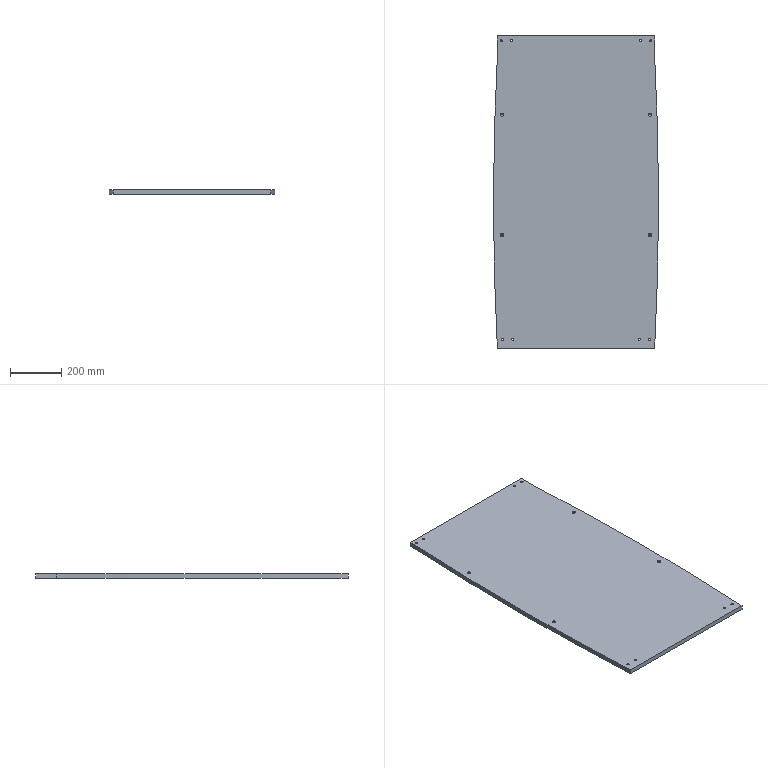Part | STEP file | DECAK 601 | 1 solid | 24 faces | box 645 x 1220 x 18 mm | volume 13904736 mm3 | cylinder 14 | plane 6 | cone 4 | commonest cylinder face diameters 8.5 x8 6.6 x4 21675 x2